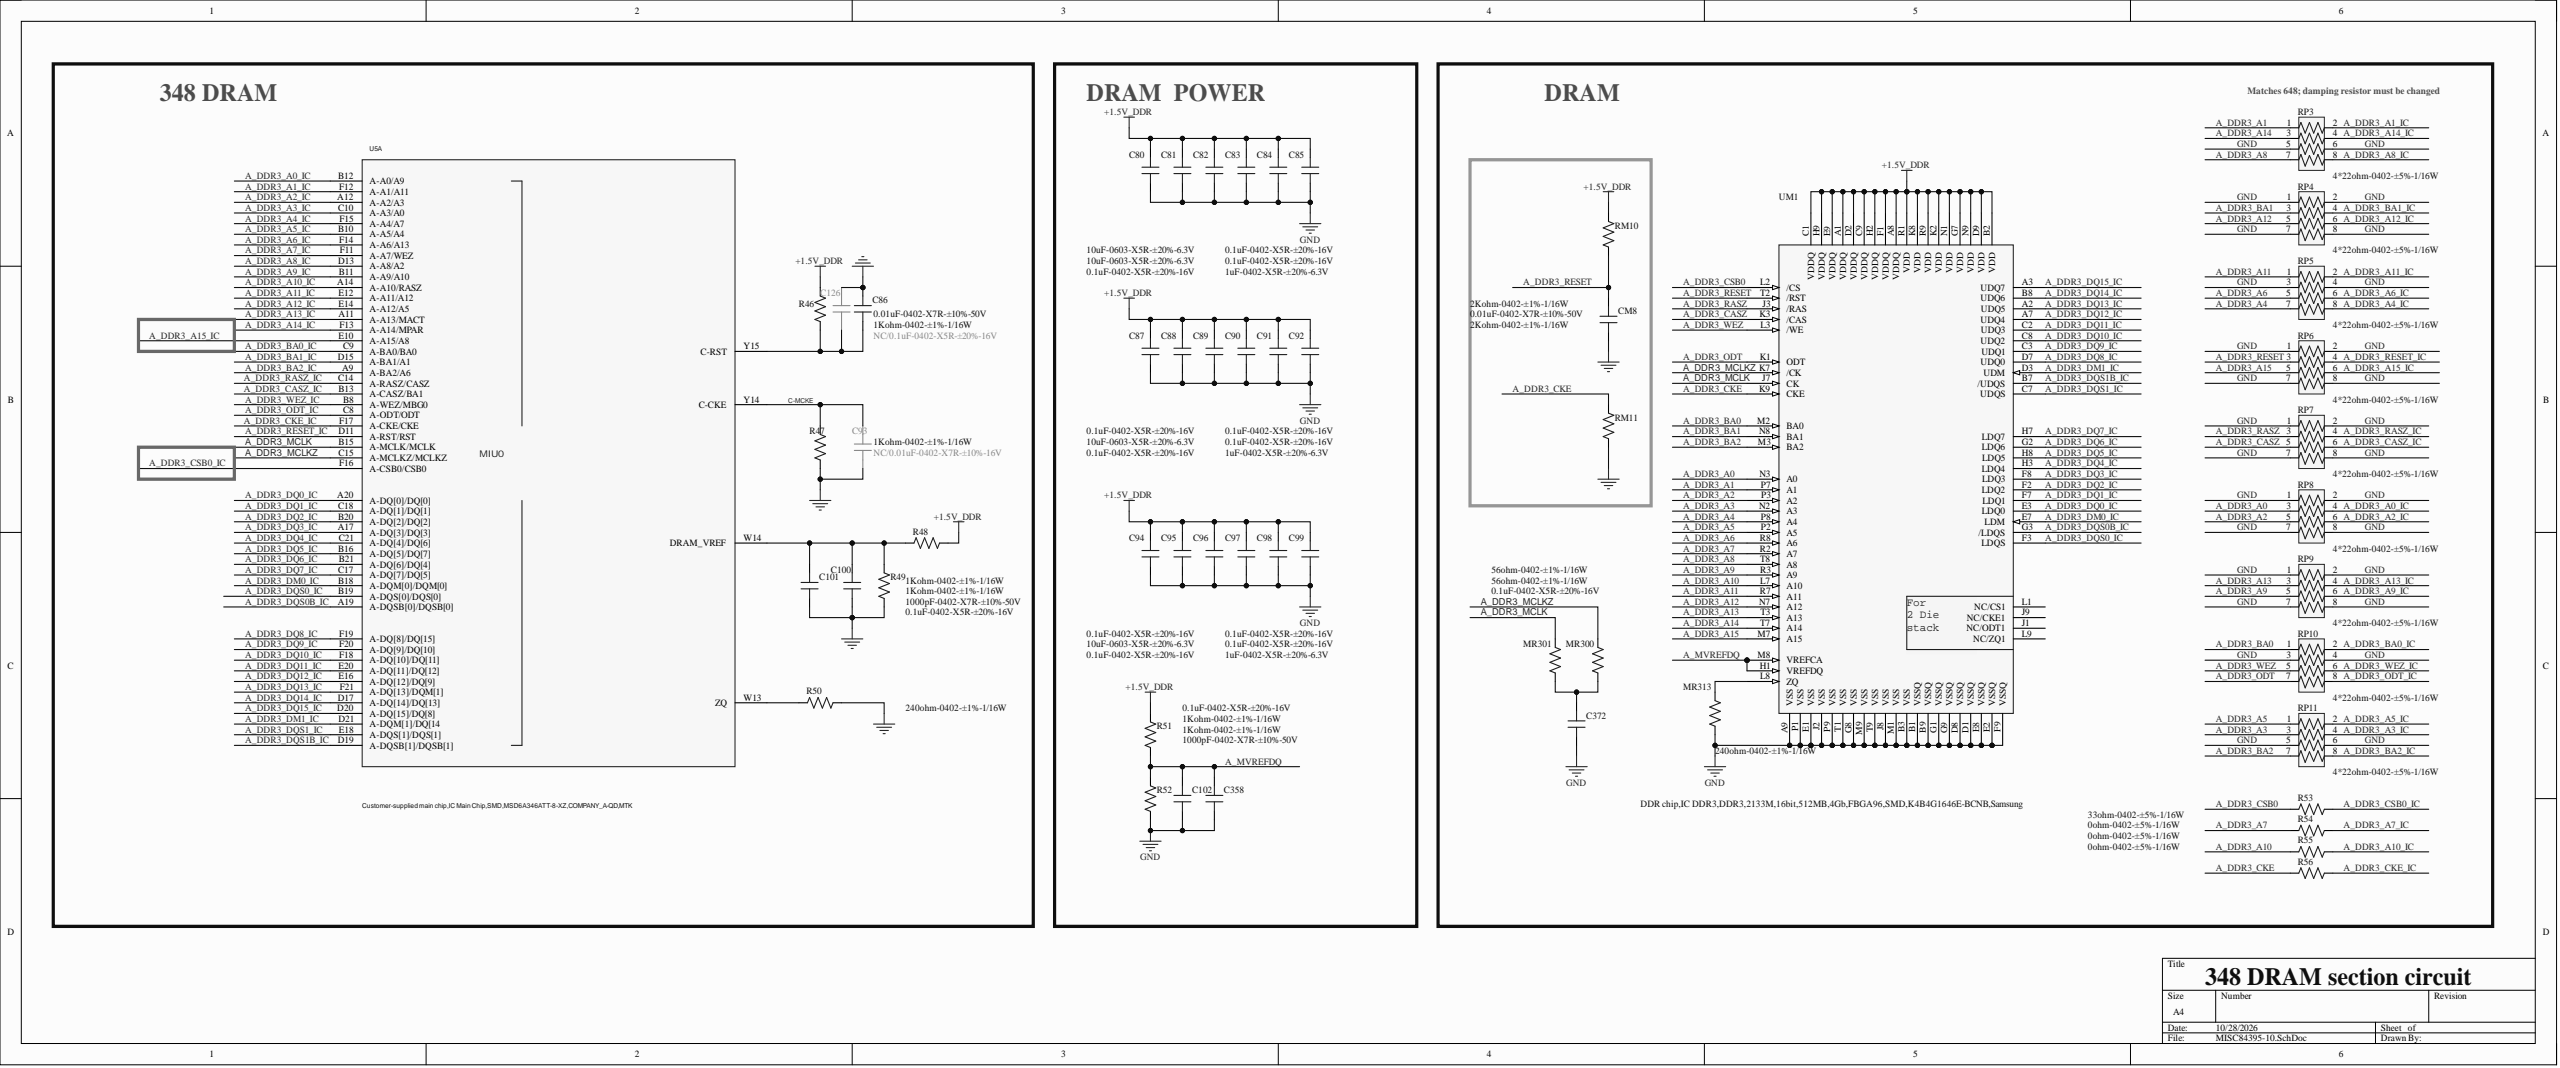Circuit board | Altium Designer | 951 parts | 509 nets | one sheet of the schematic
Parts on this sheet (reference | value | footprint):
C80 | 10uF-0603-X5R-±20%-6.3V | C0603
C81 | 10uF-0603-X5R-±20%-6.3V | C0603
C82 | 0.1uF-0402-X5R-±20%-16V | C0402
C83 | 0.1uF-0402-X5R-±20%-16V | C0402
C84 | 0.1uF-0402-X5R-±20%-16V | C0402
C85 | 1uF-0402-X5R-±20%-6.3V | C0402
C86 | 0.01uF-0402-X7R-±10%-50V | C0402
C87 | 10uF-0603-X5R-±20%-6.3V | C0603
C88 | 0.1uF-0402-X5R-±20%-16V | C0402
C89 | 0.1uF-0402-X5R-±20%-16V | C0402
C90 | 0.1uF-0402-X5R-±20%-16V | C0402
C91 | 0.1uF-0402-X5R-±20%-16V | C0402
C92 | 1uF-0402-X5R-±20%-6.3V | C0402
C93 | NC/0.01uF-0402-X7R-±10%-16V | C0402
C94 | 10uF-0603-X5R-±20%-6.3V | C0603
C95 | 0.1uF-0402-X5R-±20%-16V | C0402
C96 | 0.1uF-0402-X5R-±20%-16V | C0402
C97 | 0.1uF-0402-X5R-±20%-16V | C0402
C98 | 0.1uF-0402-X5R-±20%-16V | C0402
C99 | 1uF-0402-X5R-±20%-6.3V | C0402
C100 | 0.1uF-0402-X5R-±20%-16V | C0402
C101 | 1000pF-0402-X7R-±10%-50V | C0402
C102 | 1000pF-0402-X7R-±10%-50V | C0402
C126 | NC/0.1uF-0402-X5R-±20%-16V | C0402
C358 | 0.1uF-0402-X5R-±20%-16V | C0402
C372 | 0.1uF-0402-X5R-±20%-16V | C0402
CM8 | 0.01uF-0402-X7R-±10%-50V | C0402
MR300 | 56ohm-0402-±1%-1/16W | R0402
MR301 | 56ohm-0402-±1%-1/16W | R0402
MR313 | 240ohm-0402-±1%-1/16W | R0402
R46 | 1Kohm-0402-±1%-1/16W | R0402
R47 | 1Kohm-0402-±1%-1/16W | R0402
R48 | 1Kohm-0402-±1%-1/16W | R0402
R49 | 1Kohm-0402-±1%-1/16W | R0402
R50 | 240ohm-0402-±1%-1/16W | R0402
R51 | 1Kohm-0402-±1%-1/16W | R0402
R52 | 1Kohm-0402-±1%-1/16W | R0402
R53 | 33ohm-0402-±5%-1/16W | R0402
R54 | 0ohm-0402-±5%-1/16W | R0402
R55 | 0ohm-0402-±5%-1/16W | R0402
R56 | 0ohm-0402-±5%-1/16W | R0402
RM10 | 2Kohm-0402-±1%-1/16W | R0402
RM11 | 2Kohm-0402-±1%-1/16W | R0402
RP3 | 4*22ohm-0402-±5%-1/16W | RA0402
RP4 | 4*22ohm-0402-±5%-1/16W | RA0402
RP5 | 4*22ohm-0402-±5%-1/16W | RA0402
RP6 | 4*22ohm-0402-±5%-1/16W | RA0402
RP7 | 4*22ohm-0402-±5%-1/16W | RA0402
RP8 | 4*22ohm-0402-±5%-1/16W | RA0402
RP9 | 4*22ohm-0402-±5%-1/16W | RA0402
RP10 | 4*22ohm-0402-±5%-1/16W | RA0402
RP11 | 4*22ohm-0402-±5%-1/16W | RA0402
U5 | Customer-supplied main chip,IC Main Chip,SMD,MSD6A346ATT-8-XZ,COMPANY_A-QD,MTK | BGA406/0.8
UM1 | DDR chip,IC DDR3,DDR3,2133M,16bit,512MB,4Gb,FBGA96,SMD,K4B4G1646E-BCNB,Samsung | BGA96/0.8-1
Nets of these parts (net: part-pin ...):
NetR50_1: R50-1 U5-W13
NetMR313_2: MR313-2 UM1-L8
NetC372_2: C372-2 MR300-1 MR301-1
NetC100_2: C100-2 C101-1 R48-2 R49-1 U5-W14
NetC86_1: C86-1 C126-1 R46-1 U5-Y15
GND: C80-1 C81-1 C82-1 C83-1 C84-1 C85-1 C86-2 C87-1 C88-1 C89-1 C90-1 C91-1 C92-1 C93-1 C94-1 C95-1 C96-1 C97-1 C98-1 C99-1 C100-1 C101-2 C102-2 C126-2 C358-1 C372-1 CM8-1 MR313-1 R47-1 R49-2 R50-2 R52-1 RM11-1 RP3-5 RP3-6 RP4-1 RP4-2 RP4-7 RP4-8 RP5-3 RP5-4 RP6-1 RP6-2 RP6-7 RP6-8 RP7-1 RP7-2 RP7-7 RP7-8 RP8-1 RP8-2 RP8-7 RP8-8 RP9-1 RP9-2 RP9-7 RP9-8 RP10-3 RP10-4 RP11-5 RP11-6 U5-A8 U5-B7 U5-B9 U5-C3 U5-D7 U5-D8 U5-D9 U5-E1 U5-E7 U5-F7 U5-F8 U5-F9 U5-G7 U5-G8 U5-G9 U5-H7 U5-H8 U5-J3 U5-K8 U5-L8 U5-L9 U5-M1 U5-M7 U5-M8 U5-M9 U5-N7 U5-N8 U5-N9 U5-P7 U5-P8 U5-R7 U5-R9 UM1-A9 UM1-B1 UM1-B3 UM1-B9 UM1-D1 UM1-D8 UM1-E1 UM1-E2 UM1-E8 UM1-F9 UM1-G1 UM1-G8 UM1-G9 UM1-J2 UM1-J8 UM1-M1 UM1-M9 UM1-P1 UM1-P9 UM1-T1 UM1-T9
C-MCKE: C93-2 R47-2 U5-Y14
A_MVREFDQ: C102-1 C358-2 R51-1 R52-2 UM1-H1 UM1-M8
A_DDR3_WEZ_IC: RP10-6 U5-B8
A_DDR3_WEZ: RP10-5 UM1-L3
A_DDR3_RESET_IC: RP6-4 U5-D11
A_DDR3_RESET: CM8-2 RM10-1 RP6-3 UM1-T2
A_DDR3_RASZ_IC: RP7-4 U5-C14
A_DDR3_RASZ: RP7-3 UM1-J3
A_DDR3_ODT_IC: RP10-8 U5-C8
A_DDR3_ODT: RP10-7 UM1-K1
A_DDR3_MCLKZ: MR300-2 U5-C15 UM1-K7
A_DDR3_MCLK: MR301-2 U5-B15 UM1-J7
A_DDR3_DQS1B_IC: U5-D19 UM1-B7
A_DDR3_DQS1_IC: U5-E18 UM1-C7
A_DDR3_DQS0B_IC: U5-A19 UM1-G3
A_DDR3_DQS0_IC: U5-B19 UM1-F3
A_DDR3_DQ15_IC: U5-D20 UM1-A3
A_DDR3_DQ14_IC: U5-D17 UM1-B8
A_DDR3_DQ13_IC: U5-F21 UM1-A2
A_DDR3_DQ12_IC: U5-E16 UM1-A7
A_DDR3_DQ11_IC: U5-E20 UM1-C2
A_DDR3_DQ10_IC: U5-F18 UM1-C8
A_DDR3_DQ9_IC: U5-F20 UM1-C3
A_DDR3_DQ8_IC: U5-F19 UM1-D7
A_DDR3_DQ7_IC: U5-C17 UM1-H7
A_DDR3_DQ6_IC: U5-B21 UM1-G2
A_DDR3_DQ5_IC: U5-B16 UM1-H8
A_DDR3_DQ4_IC: U5-C21 UM1-H3
A_DDR3_DQ3_IC: U5-A17 UM1-F8
A_DDR3_DQ2_IC: U5-B20 UM1-F2
A_DDR3_DQ1_IC: U5-C18 UM1-F7
A_DDR3_DQ0_IC: U5-A20 UM1-E3
A_DDR3_DM1_IC: U5-D21 UM1-D3
A_DDR3_DM0_IC: U5-B18 UM1-E7
A_DDR3_CSB0_IC: R53-2 U5-F16
A_DDR3_CSB0: R53-1 UM1-L2
A_DDR3_CKE_IC: R56-2 U5-F17
A_DDR3_CKE: R56-1 RM11-2 UM1-K9
A_DDR3_CASZ_IC: RP7-6 U5-B13
A_DDR3_CASZ: RP7-5 UM1-K3
A_DDR3_BA2_IC: RP11-8 U5-A9
A_DDR3_BA2: RP11-7 UM1-M3
A_DDR3_BA1_IC: RP4-4 U5-D15
A_DDR3_BA1: RP4-3 UM1-N8
A_DDR3_BA0_IC: RP10-2 U5-C9
A_DDR3_BA0: RP10-1 UM1-M2
A_DDR3_A15_IC: RP6-6 U5-E10
A_DDR3_A15: RP6-5 UM1-M7
A_DDR3_A14_IC: RP3-4 U5-F13
A_DDR3_A14: RP3-3 UM1-T7
A_DDR3_A13_IC: RP9-4 U5-A11
A_DDR3_A13: RP9-3 UM1-T3
A_DDR3_A12_IC: RP4-6 U5-E14
A_DDR3_A12: RP4-5 UM1-N7
A_DDR3_A11_IC: RP5-2 U5-E12
A_DDR3_A11: RP5-1 UM1-R7
A_DDR3_A10_IC: R55-2 U5-A14
A_DDR3_A10: R55-1 UM1-L7
A_DDR3_A9_IC: RP9-6 U5-B11
A_DDR3_A9: RP9-5 UM1-R3
A_DDR3_A8_IC: RP3-8 U5-D13
A_DDR3_A8: RP3-7 UM1-T8
A_DDR3_A7_IC: R54-2 U5-F11
A_DDR3_A7: R54-1 UM1-R2
A_DDR3_A6_IC: RP5-6 U5-F14
A_DDR3_A6: RP5-5 UM1-R8
A_DDR3_A5_IC: RP11-2 U5-B10
A_DDR3_A5: RP11-1 UM1-P2
A_DDR3_A4_IC: RP5-8 U5-F15
A_DDR3_A4: RP5-7 UM1-P8
A_DDR3_A3_IC: RP11-4 U5-C10
A_DDR3_A3: RP11-3 UM1-N2
A_DDR3_A2_IC: RP8-6 U5-A12
A_DDR3_A2: RP8-5 UM1-P3
A_DDR3_A1_IC: RP3-2 U5-F12
A_DDR3_A1: RP3-1 UM1-P7
A_DDR3_A0_IC: RP8-4 U5-B12
A_DDR3_A0: RP8-3 UM1-N3
+1.5V_DDR: C80-2 C81-2 C82-2 C83-2 C84-2 C85-2 C87-2 C88-2 C89-2 C90-2 C91-2 C92-2 C94-2 C95-2 C96-2 C97-2 C98-2 C99-2 R46-2 R48-1 R51-2 RM10-2 U5-K9 UM1-A1 UM1-A8 UM1-B2 UM1-C1 UM1-C9 UM1-D2 UM1-D9 UM1-E9 UM1-F1 UM1-G7 UM1-H2 UM1-H9 UM1-K2 UM1-K8 UM1-N1 UM1-N9 UM1-R1 UM1-R9